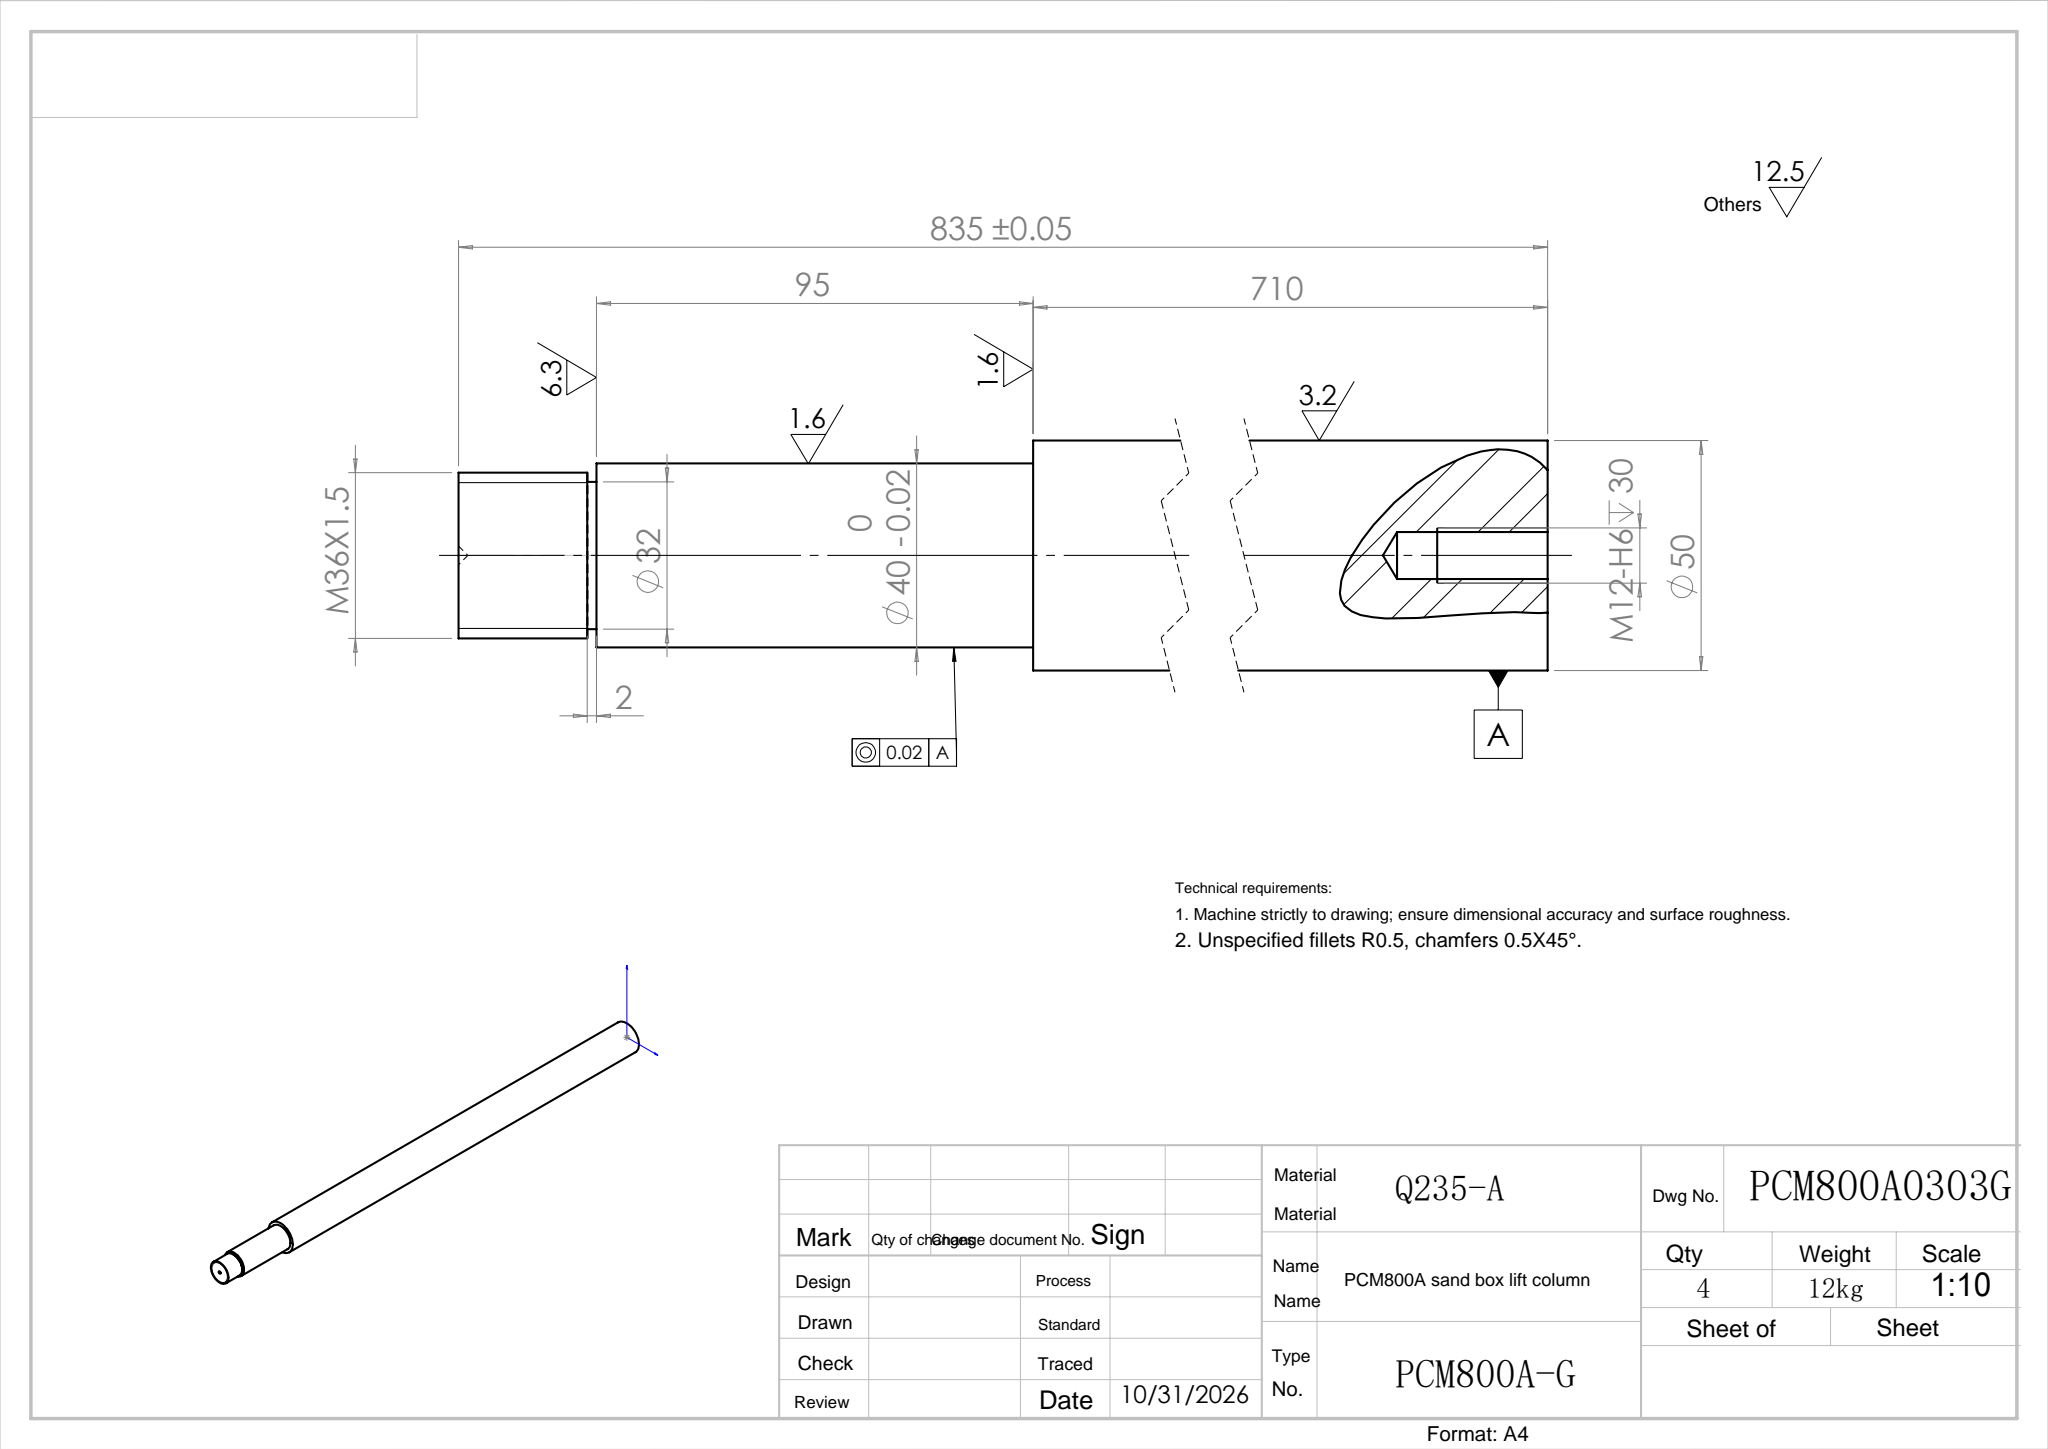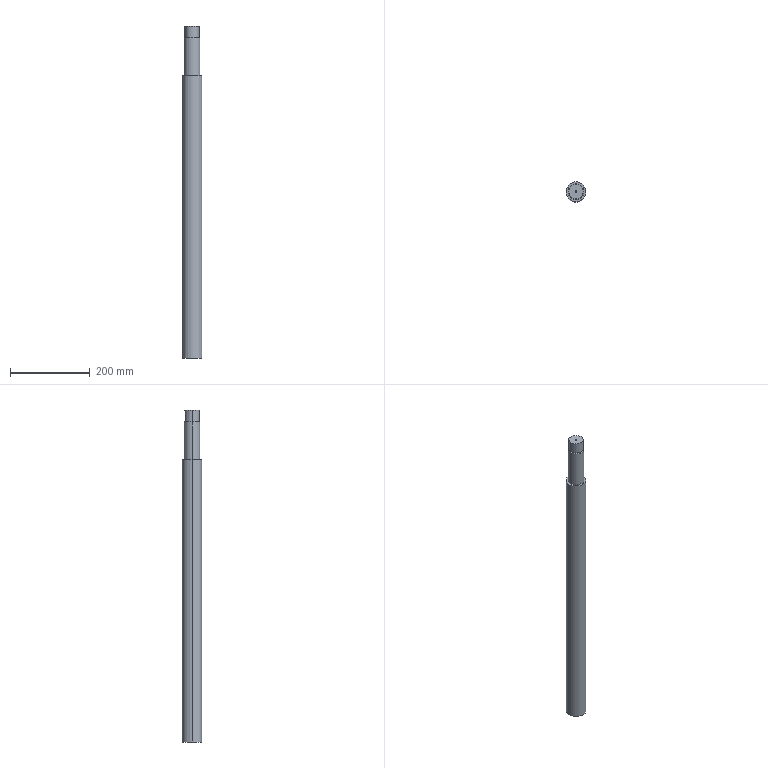Part | SolidWorks | features Boss 2, Extrusion 1, HoleWzd 1, ICE 1, RevCut 1 | 1 solid | 19 faces | box 50 x 50 x 835 mm | volume 1540803 mm3 | cylinder 10 | plane 5 | cone 4 | commonest cylinder face diameters 10.2 x2 32 x2 36 x2 40 x2 50 x2
STEP:
#1=CARTESIAN_POINT('',(18.,0.,835.));
#2=VERTEX_POINT('',#1);
#3=CARTESIAN_POINT('',(-18.,0.,835.));
#4=VERTEX_POINT('',#3);
#5=CARTESIAN_POINT('',(0.,0.,835.));
#6=DIRECTION('',(0.,0.,1.));
#7=DIRECTION('',(1.,0.,0.));
#8=AXIS2_PLACEMENT_3D('',#5,#6,#7);
#9=CIRCLE('',#8,18.);
#10=EDGE_CURVE('',#2,#4,#9,.T.);
#11=ORIENTED_EDGE('',*,*,#10,.F.);
#12=CARTESIAN_POINT('',(18.,0.,807.));
#13=VERTEX_POINT('',#12);
#14=CARTESIAN_POINT('',(18.,0.,835.));
#15=DIRECTION('',(0.,0.,-1.));
#16=VECTOR('',#15,1000.);
#17=LINE('',#14,#16);
#18=EDGE_CURVE('',#2,#13,#17,.T.);
#19=ORIENTED_EDGE('',*,*,#18,.T.);
#20=CARTESIAN_POINT('',(-18.,0.,807.));
#21=VERTEX_POINT('',#20);
#22=CARTESIAN_POINT('',(0.,0.,807.));
#23=DIRECTION('',(0.,0.,1.));
#24=DIRECTION('',(1.,0.,0.));
#25=AXIS2_PLACEMENT_3D('',#22,#23,#24);
#26=CIRCLE('',#25,18.);
#27=EDGE_CURVE('',#13,#21,#26,.T.);
#28=ORIENTED_EDGE('',*,*,#27,.T.);
#29=CARTESIAN_POINT('',(-18.,0.,835.));
#30=DIRECTION('',(0.,0.,-1.));
#31=VECTOR('',#30,1000.);
#32=LINE('',#29,#31);
#33=EDGE_CURVE('',#4,#21,#32,.T.);
#34=ORIENTED_EDGE('',*,*,#33,.F.);
#35=EDGE_LOOP('',(#11,#19,#28,#34));
#36=FACE_OUTER_BOUND('',#35,.T.);
#37=CARTESIAN_POINT('',(0.,0.,835.));
#38=DIRECTION('',(0.,0.,-1.));
#39=DIRECTION('',(-1.,0.,0.));
#40=AXIS2_PLACEMENT_3D('',#37,#38,#39);
#41=CYLINDRICAL_SURFACE('',#40,18.);
#42=ADVANCED_FACE('',(#36),#41,.T.);
#43=CARTESIAN_POINT('',(0.,0.,833.));
#44=VERTEX_POINT('',#43);
#45=CARTESIAN_POINT('',(2.,0.,835.));
#46=VERTEX_POINT('',#45);
#47=CARTESIAN_POINT('',(0.,0.,833.));
#48=DIRECTION('',(0.7071,0.,0.7071));
#49=VECTOR('',#48,1000.);
#50=LINE('',#47,#49);
#51=EDGE_CURVE('',#44,#46,#50,.T.);
#52=ORIENTED_EDGE('',*,*,#51,.F.);
#53=CARTESIAN_POINT('',(-2.,0.,835.));
#54=VERTEX_POINT('',#53);
#55=CARTESIAN_POINT('',(0.,0.,833.));
#56=DIRECTION('',(-0.7071,0.,0.7071));
#57=VECTOR('',#56,1000.);
#58=LINE('',#55,#57);
#59=EDGE_CURVE('',#44,#54,#58,.T.);
#60=ORIENTED_EDGE('',*,*,#59,.T.);
#61=CARTESIAN_POINT('',(0.,0.,835.));
#62=DIRECTION('',(0.,0.,1.));
#63=DIRECTION('',(1.,0.,0.));
#64=AXIS2_PLACEMENT_3D('',#61,#62,#63);
#65=CIRCLE('',#64,2.);
#66=EDGE_CURVE('',#54,#46,#65,.T.);
#67=ORIENTED_EDGE('',*,*,#66,.T.);
#68=EDGE_LOOP('',(#52,#60,#67));
#69=FACE_OUTER_BOUND('',#68,.T.);
#70=CARTESIAN_POINT('',(0.,0.,1833.));
#71=DIRECTION('',(0.,0.,1.));
#72=DIRECTION('',(1.,0.,0.));
#73=AXIS2_PLACEMENT_3D('',#70,#71,#72);
#74=CONICAL_SURFACE('',#73,1000.,0.7854);
#75=ADVANCED_FACE('',(#69),#74,.F.);
#76=CARTESIAN_POINT('',(16.,0.,807.));
#77=VERTEX_POINT('',#76);
#78=CARTESIAN_POINT('',(-16.,0.,807.));
#79=VERTEX_POINT('',#78);
#80=CARTESIAN_POINT('',(0.,0.,807.));
#81=DIRECTION('',(0.,0.,1.));
#82=DIRECTION('',(1.,0.,0.));
#83=AXIS2_PLACEMENT_3D('',#80,#81,#82);
#84=CIRCLE('',#83,16.);
#85=EDGE_CURVE('',#77,#79,#84,.T.);
#86=ORIENTED_EDGE('',*,*,#85,.F.);
#87=CARTESIAN_POINT('',(16.,0.,805.));
#88=VERTEX_POINT('',#87);
#89=CARTESIAN_POINT('',(16.,0.,807.));
#90=DIRECTION('',(0.,0.,-1.));
#91=VECTOR('',#90,1000.);
#92=LINE('',#89,#91);
#93=EDGE_CURVE('',#77,#88,#92,.T.);
#94=ORIENTED_EDGE('',*,*,#93,.T.);
#95=CARTESIAN_POINT('',(-16.,0.,805.));
#96=VERTEX_POINT('',#95);
#97=CARTESIAN_POINT('',(0.,0.,805.));
#98=DIRECTION('',(0.,0.,1.));
#99=DIRECTION('',(1.,0.,0.));
#100=AXIS2_PLACEMENT_3D('',#97,#98,#99);
#101=CIRCLE('',#100,16.);
#102=EDGE_CURVE('',#88,#96,#101,.T.);
#103=ORIENTED_EDGE('',*,*,#102,.T.);
#104=CARTESIAN_POINT('',(-16.,0.,807.));
#105=DIRECTION('',(0.,0.,-1.));
#106=VECTOR('',#105,1000.);
#107=LINE('',#104,#106);
#108=EDGE_CURVE('',#79,#96,#107,.T.);
#109=ORIENTED_EDGE('',*,*,#108,.F.);
#110=EDGE_LOOP('',(#86,#94,#103,#109));
#111=FACE_OUTER_BOUND('',#110,.T.);
#112=CARTESIAN_POINT('',(0.,0.,807.));
#113=DIRECTION('',(0.,0.,-1.));
#114=DIRECTION('',(-1.,0.,0.));
#115=AXIS2_PLACEMENT_3D('',#112,#113,#114);
#116=CYLINDRICAL_SURFACE('',#115,16.);
#117=ADVANCED_FACE('',(#111),#116,.T.);
#118=CARTESIAN_POINT('',(5.1,0.,32.75));
#119=VERTEX_POINT('',#118);
#120=CARTESIAN_POINT('',(-5.1,0.,32.75));
#121=VERTEX_POINT('',#120);
#122=CARTESIAN_POINT('',(0.,0.,32.75));
#123=DIRECTION('',(0.,0.,-1.));
#124=DIRECTION('',(-1.,0.,0.));
#125=AXIS2_PLACEMENT_3D('',#122,#123,#124);
#126=CIRCLE('',#125,5.1);
#127=EDGE_CURVE('',#119,#121,#126,.T.);
#128=ORIENTED_EDGE('',*,*,#127,.F.);
#129=CARTESIAN_POINT('',(5.1,0.,0.));
#130=VERTEX_POINT('',#129);
#131=CARTESIAN_POINT('',(5.1,0.,0.));
#132=DIRECTION('',(0.,0.,-1.));
#133=VECTOR('',#132,1000.);
#134=LINE('',#131,#133);
#135=EDGE_CURVE('',#119,#130,#134,.T.);
#136=ORIENTED_EDGE('',*,*,#135,.T.);
#137=CARTESIAN_POINT('',(-5.1,0.,0.));
#138=VERTEX_POINT('',#137);
#139=CARTESIAN_POINT('',(0.,0.,0.));
#140=DIRECTION('',(0.,0.,-1.));
#141=DIRECTION('',(-1.,0.,0.));
#142=AXIS2_PLACEMENT_3D('',#139,#140,#141);
#143=CIRCLE('',#142,5.1);
#144=EDGE_CURVE('',#130,#138,#143,.T.);
#145=ORIENTED_EDGE('',*,*,#144,.T.);
#146=CARTESIAN_POINT('',(-5.1,0.,0.));
#147=DIRECTION('',(0.,0.,-1.));
#148=VECTOR('',#147,1000.);
#149=LINE('',#146,#148);
#150=EDGE_CURVE('',#121,#138,#149,.T.);
#151=ORIENTED_EDGE('',*,*,#150,.F.);
#152=EDGE_LOOP('',(#128,#136,#145,#151));
#153=FACE_OUTER_BOUND('',#152,.T.);
#154=CARTESIAN_POINT('',(0.,0.,0.));
#155=DIRECTION('',(0.,0.,-1.));
#156=DIRECTION('',(-1.,0.,0.));
#157=AXIS2_PLACEMENT_3D('',#154,#155,#156);
#158=CYLINDRICAL_SURFACE('',#157,5.1);
#159=ADVANCED_FACE('',(#153),#158,.F.);
#160=CARTESIAN_POINT('',(0.,0.,35.814));
#161=VERTEX_POINT('',#160);
#162=CARTESIAN_POINT('',(-5.1,0.,32.75));
#163=DIRECTION('',(-0.8572,0.,-0.515));
#164=VECTOR('',#163,1000.);
#165=LINE('',#162,#164);
#166=EDGE_CURVE('',#161,#121,#165,.T.);
#167=ORIENTED_EDGE('',*,*,#166,.F.);
#168=CARTESIAN_POINT('',(5.1,0.,32.75));
#169=DIRECTION('',(0.8572,0.,-0.515));
#170=VECTOR('',#169,1000.);
#171=LINE('',#168,#170);
#172=EDGE_CURVE('',#161,#119,#171,.T.);
#173=ORIENTED_EDGE('',*,*,#172,.T.);
#174=ORIENTED_EDGE('',*,*,#127,.T.);
#175=EDGE_LOOP('',(#167,#173,#174));
#176=FACE_OUTER_BOUND('',#175,.T.);
#177=CARTESIAN_POINT('',(0.,0.,32.75));
#178=DIRECTION('',(0.,0.,-1.));
#179=DIRECTION('',(-1.,0.,0.));
#180=AXIS2_PLACEMENT_3D('',#177,#178,#179);
#181=CONICAL_SURFACE('',#180,5.1,1.03);
#182=ADVANCED_FACE('',(#176),#181,.F.);
#183=CARTESIAN_POINT('',(20.,0.,805.));
#184=VERTEX_POINT('',#183);
#185=CARTESIAN_POINT('',(-20.,0.,805.));
#186=VERTEX_POINT('',#185);
#187=CARTESIAN_POINT('',(0.,0.,805.));
#188=DIRECTION('',(0.,0.,1.));
#189=DIRECTION('',(1.,0.,0.));
#190=AXIS2_PLACEMENT_3D('',#187,#188,#189);
#191=CIRCLE('',#190,20.);
#192=EDGE_CURVE('',#184,#186,#191,.T.);
#193=ORIENTED_EDGE('',*,*,#192,.F.);
#194=CARTESIAN_POINT('',(20.,0.,710.));
#195=VERTEX_POINT('',#194);
#196=CARTESIAN_POINT('',(20.,0.,805.));
#197=DIRECTION('',(0.,0.,-1.));
#198=VECTOR('',#197,1000.);
#199=LINE('',#196,#198);
#200=EDGE_CURVE('',#184,#195,#199,.T.);
#201=ORIENTED_EDGE('',*,*,#200,.T.);
#202=CARTESIAN_POINT('',(-20.,0.,710.));
#203=VERTEX_POINT('',#202);
#204=CARTESIAN_POINT('',(0.,0.,710.));
#205=DIRECTION('',(0.,0.,1.));
#206=DIRECTION('',(1.,0.,0.));
#207=AXIS2_PLACEMENT_3D('',#204,#205,#206);
#208=CIRCLE('',#207,20.);
#209=EDGE_CURVE('',#195,#203,#208,.T.);
#210=ORIENTED_EDGE('',*,*,#209,.T.);
#211=CARTESIAN_POINT('',(-20.,0.,805.));
#212=DIRECTION('',(0.,0.,-1.));
#213=VECTOR('',#212,1000.);
#214=LINE('',#211,#213);
#215=EDGE_CURVE('',#186,#203,#214,.T.);
#216=ORIENTED_EDGE('',*,*,#215,.F.);
#217=EDGE_LOOP('',(#193,#201,#210,#216));
#218=FACE_OUTER_BOUND('',#217,.T.);
#219=CARTESIAN_POINT('',(0.,0.,805.));
#220=DIRECTION('',(0.,0.,-1.));
#221=DIRECTION('',(-1.,0.,0.));
#222=AXIS2_PLACEMENT_3D('',#219,#220,#221);
#223=CYLINDRICAL_SURFACE('',#222,20.);
#224=ADVANCED_FACE('',(#218),#223,.T.);
#225=CARTESIAN_POINT('',(25.,0.,710.));
#226=VERTEX_POINT('',#225);
#227=CARTESIAN_POINT('',(-25.,0.,710.));
#228=VERTEX_POINT('',#227);
#229=CARTESIAN_POINT('',(0.,0.,710.));
#230=DIRECTION('',(0.,0.,1.));
#231=DIRECTION('',(1.,0.,0.));
#232=AXIS2_PLACEMENT_3D('',#229,#230,#231);
#233=CIRCLE('',#232,25.);
#234=EDGE_CURVE('',#226,#228,#233,.T.);
#235=ORIENTED_EDGE('',*,*,#234,.F.);
#236=CARTESIAN_POINT('',(25.,0.,0.));
#237=VERTEX_POINT('',#236);
#238=CARTESIAN_POINT('',(25.,0.,710.));
#239=DIRECTION('',(0.,0.,-1.));
#240=VECTOR('',#239,1000.);
#241=LINE('',#238,#240);
#242=EDGE_CURVE('',#226,#237,#241,.T.);
#243=ORIENTED_EDGE('',*,*,#242,.T.);
#244=CARTESIAN_POINT('',(-25.,0.,0.));
#245=VERTEX_POINT('',#244);
#246=CARTESIAN_POINT('',(0.,0.,0.));
#247=DIRECTION('',(0.,0.,1.));
#248=DIRECTION('',(1.,0.,0.));
#249=AXIS2_PLACEMENT_3D('',#246,#247,#248);
#250=CIRCLE('',#249,25.);
#251=EDGE_CURVE('',#237,#245,#250,.T.);
#252=ORIENTED_EDGE('',*,*,#251,.T.);
#253=CARTESIAN_POINT('',(-25.,0.,710.));
#254=DIRECTION('',(0.,0.,-1.));
#255=VECTOR('',#254,1000.);
#256=LINE('',#253,#255);
#257=EDGE_CURVE('',#228,#245,#256,.T.);
#258=ORIENTED_EDGE('',*,*,#257,.F.);
#259=EDGE_LOOP('',(#235,#243,#252,#258));
#260=FACE_OUTER_BOUND('',#259,.T.);
#261=CARTESIAN_POINT('',(0.,0.,710.));
#262=DIRECTION('',(0.,0.,-1.));
#263=DIRECTION('',(-1.,0.,0.));
#264=AXIS2_PLACEMENT_3D('',#261,#262,#263);
#265=CYLINDRICAL_SURFACE('',#264,25.);
#266=ADVANCED_FACE('',(#260),#265,.T.);
#267=CARTESIAN_POINT('',(0.,0.,805.));
#268=DIRECTION('',(0.,0.,1.));
#269=DIRECTION('',(1.,0.,0.));
#270=AXIS2_PLACEMENT_3D('',#267,#268,#269);
#271=CIRCLE('',#270,20.);
#272=EDGE_CURVE('',#186,#184,#271,.T.);
#273=ORIENTED_EDGE('',*,*,#272,.T.);
#274=ORIENTED_EDGE('',*,*,#192,.T.);
#275=EDGE_LOOP('',(#273,#274));
#276=FACE_OUTER_BOUND('',#275,.T.);
#277=CARTESIAN_POINT('',(0.,0.,805.));
#278=DIRECTION('',(0.,0.,1.));
#279=DIRECTION('',(1.,0.,0.));
#280=AXIS2_PLACEMENT_3D('',#277,#278,#279);
#281=CIRCLE('',#280,16.);
#282=EDGE_CURVE('',#96,#88,#281,.T.);
#283=ORIENTED_EDGE('',*,*,#282,.F.);
#284=ORIENTED_EDGE('',*,*,#102,.F.);
#285=EDGE_LOOP('',(#283,#284));
#286=FACE_BOUND('',#285,.T.);
#287=CARTESIAN_POINT('',(0.,0.,805.));
#288=DIRECTION('',(0.,0.,1.));
#289=DIRECTION('',(1.,0.,0.));
#290=AXIS2_PLACEMENT_3D('',#287,#288,#289);
#291=PLANE('',#290);
#292=ADVANCED_FACE('',(#276,#286),#291,.T.);
#293=CARTESIAN_POINT('',(0.,0.,710.));
#294=DIRECTION('',(0.,0.,1.));
#295=DIRECTION('',(1.,0.,0.));
#296=AXIS2_PLACEMENT_3D('',#293,#294,#295);
#297=CIRCLE('',#296,25.);
#298=EDGE_CURVE('',#228,#226,#297,.T.);
#299=ORIENTED_EDGE('',*,*,#298,.T.);
#300=ORIENTED_EDGE('',*,*,#234,.T.);
#301=EDGE_LOOP('',(#299,#300));
#302=FACE_OUTER_BOUND('',#301,.T.);
#303=CARTESIAN_POINT('',(0.,0.,710.));
#304=DIRECTION('',(0.,0.,1.));
#305=DIRECTION('',(1.,0.,0.));
#306=AXIS2_PLACEMENT_3D('',#303,#304,#305);
#307=CIRCLE('',#306,20.);
#308=EDGE_CURVE('',#203,#195,#307,.T.);
#309=ORIENTED_EDGE('',*,*,#308,.F.);
#310=ORIENTED_EDGE('',*,*,#209,.F.);
#311=EDGE_LOOP('',(#309,#310));
#312=FACE_BOUND('',#311,.T.);
#313=CARTESIAN_POINT('',(0.,0.,710.));
#314=DIRECTION('',(0.,0.,1.));
#315=DIRECTION('',(1.,0.,0.));
#316=AXIS2_PLACEMENT_3D('',#313,#314,#315);
#317=PLANE('',#316);
#318=ADVANCED_FACE('',(#302,#312),#317,.T.);
#319=ORIENTED_EDGE('',*,*,#242,.F.);
#320=ORIENTED_EDGE('',*,*,#298,.F.);
#321=ORIENTED_EDGE('',*,*,#257,.T.);
#322=CARTESIAN_POINT('',(0.,0.,0.));
#323=DIRECTION('',(0.,0.,1.));
#324=DIRECTION('',(1.,0.,0.));
#325=AXIS2_PLACEMENT_3D('',#322,#323,#324);
#326=CIRCLE('',#325,25.);
#327=EDGE_CURVE('',#245,#237,#326,.T.);
#328=ORIENTED_EDGE('',*,*,#327,.T.);
#329=EDGE_LOOP('',(#319,#320,#321,#328));
#330=FACE_OUTER_BOUND('',#329,.T.);
#331=CARTESIAN_POINT('',(0.,0.,710.));
#332=DIRECTION('',(0.,0.,-1.));
#333=DIRECTION('',(-1.,0.,0.));
#334=AXIS2_PLACEMENT_3D('',#331,#332,#333);
#335=CYLINDRICAL_SURFACE('',#334,25.);
#336=ADVANCED_FACE('',(#330),#335,.T.);
#337=CARTESIAN_POINT('',(0.,0.,0.));
#338=DIRECTION('',(0.,0.,-1.));
#339=DIRECTION('',(-1.,0.,0.));
#340=AXIS2_PLACEMENT_3D('',#337,#338,#339);
#341=CIRCLE('',#340,5.1);
#342=EDGE_CURVE('',#138,#130,#341,.T.);
#343=ORIENTED_EDGE('',*,*,#342,.F.);
#344=ORIENTED_EDGE('',*,*,#144,.F.);
#345=EDGE_LOOP('',(#343,#344));
#346=FACE_BOUND('',#345,.T.);
#347=ORIENTED_EDGE('',*,*,#327,.F.);
#348=ORIENTED_EDGE('',*,*,#251,.F.);
#349=EDGE_LOOP('',(#347,#348));
#350=FACE_OUTER_BOUND('',#349,.T.);
#351=CARTESIAN_POINT('',(0.,0.,0.));
#352=DIRECTION('',(0.,0.,1.));
#353=DIRECTION('',(1.,0.,0.));
#354=AXIS2_PLACEMENT_3D('',#351,#352,#353);
#355=PLANE('',#354);
#356=ADVANCED_FACE('',(#346,#350),#355,.F.);
#357=ORIENTED_EDGE('',*,*,#200,.F.);
#358=ORIENTED_EDGE('',*,*,#272,.F.);
#359=ORIENTED_EDGE('',*,*,#215,.T.);
#360=ORIENTED_EDGE('',*,*,#308,.T.);
#361=EDGE_LOOP('',(#357,#358,#359,#360));
#362=FACE_OUTER_BOUND('',#361,.T.);
#363=CARTESIAN_POINT('',(0.,0.,805.));
#364=DIRECTION('',(0.,0.,-1.));
#365=DIRECTION('',(-1.,0.,0.));
#366=AXIS2_PLACEMENT_3D('',#363,#364,#365);
#367=CYLINDRICAL_SURFACE('',#366,20.);
#368=ADVANCED_FACE('',(#362),#367,.T.);
#369=ORIENTED_EDGE('',*,*,#172,.F.);
#370=ORIENTED_EDGE('',*,*,#166,.T.);
#371=CARTESIAN_POINT('',(0.,0.,32.75));
#372=DIRECTION('',(0.,0.,-1.));
#373=DIRECTION('',(-1.,0.,0.));
#374=AXIS2_PLACEMENT_3D('',#371,#372,#373);
#375=CIRCLE('',#374,5.1);
#376=EDGE_CURVE('',#121,#119,#375,.T.);
#377=ORIENTED_EDGE('',*,*,#376,.T.);
#378=EDGE_LOOP('',(#369,#370,#377));
#379=FACE_OUTER_BOUND('',#378,.T.);
#380=CARTESIAN_POINT('',(0.,0.,32.75));
#381=DIRECTION('',(0.,0.,-1.));
#382=DIRECTION('',(-1.,0.,0.));
#383=AXIS2_PLACEMENT_3D('',#380,#381,#382);
#384=CONICAL_SURFACE('',#383,5.1,1.03);
#385=ADVANCED_FACE('',(#379),#384,.F.);
#386=ORIENTED_EDGE('',*,*,#135,.F.);
#387=ORIENTED_EDGE('',*,*,#376,.F.);
#388=ORIENTED_EDGE('',*,*,#150,.T.);
#389=ORIENTED_EDGE('',*,*,#342,.T.);
#390=EDGE_LOOP('',(#386,#387,#388,#389));
#391=FACE_OUTER_BOUND('',#390,.T.);
#392=CARTESIAN_POINT('',(0.,0.,0.));
#393=DIRECTION('',(0.,0.,-1.));
#394=DIRECTION('',(-1.,0.,0.));
#395=AXIS2_PLACEMENT_3D('',#392,#393,#394);
#396=CYLINDRICAL_SURFACE('',#395,5.1);
#397=ADVANCED_FACE('',(#391),#396,.F.);
#398=CARTESIAN_POINT('',(0.,0.,807.));
#399=DIRECTION('',(0.,0.,1.));
#400=DIRECTION('',(1.,0.,0.));
#401=AXIS2_PLACEMENT_3D('',#398,#399,#400);
#402=CIRCLE('',#401,16.);
#403=EDGE_CURVE('',#79,#77,#402,.T.);
#404=ORIENTED_EDGE('',*,*,#403,.T.);
#405=ORIENTED_EDGE('',*,*,#85,.T.);
#406=EDGE_LOOP('',(#404,#405));
#407=FACE_BOUND('',#406,.T.);
#408=CARTESIAN_POINT('',(0.,0.,807.));
#409=DIRECTION('',(0.,0.,1.));
#410=DIRECTION('',(1.,0.,0.));
#411=AXIS2_PLACEMENT_3D('',#408,#409,#410);
#412=CIRCLE('',#411,18.);
#413=EDGE_CURVE('',#21,#13,#412,.T.);
#414=ORIENTED_EDGE('',*,*,#413,.F.);
#415=ORIENTED_EDGE('',*,*,#27,.F.);
#416=EDGE_LOOP('',(#414,#415));
#417=FACE_OUTER_BOUND('',#416,.T.);
#418=CARTESIAN_POINT('',(0.,0.,807.));
#419=DIRECTION('',(0.,0.,1.));
#420=DIRECTION('',(1.,0.,0.));
#421=AXIS2_PLACEMENT_3D('',#418,#419,#420);
#422=PLANE('',#421);
#423=ADVANCED_FACE('',(#407,#417),#422,.F.);
#424=ORIENTED_EDGE('',*,*,#93,.F.);
#425=ORIENTED_EDGE('',*,*,#403,.F.);
#426=ORIENTED_EDGE('',*,*,#108,.T.);
#427=ORIENTED_EDGE('',*,*,#282,.T.);
#428=EDGE_LOOP('',(#424,#425,#426,#427));
#429=FACE_OUTER_BOUND('',#428,.T.);
#430=CARTESIAN_POINT('',(0.,0.,807.));
#431=DIRECTION('',(0.,0.,-1.));
#432=DIRECTION('',(-1.,0.,0.));
#433=AXIS2_PLACEMENT_3D('',#430,#431,#432);
#434=CYLINDRICAL_SURFACE('',#433,16.);
#435=ADVANCED_FACE('',(#429),#434,.T.);
#436=ORIENTED_EDGE('',*,*,#59,.F.);
#437=ORIENTED_EDGE('',*,*,#51,.T.);
#438=CARTESIAN_POINT('',(0.,0.,835.));
#439=DIRECTION('',(0.,0.,1.));
#440=DIRECTION('',(1.,0.,0.));
#441=AXIS2_PLACEMENT_3D('',#438,#439,#440);
#442=CIRCLE('',#441,2.);
#443=EDGE_CURVE('',#46,#54,#442,.T.);
#444=ORIENTED_EDGE('',*,*,#443,.T.);
#445=EDGE_LOOP('',(#436,#437,#444));
#446=FACE_OUTER_BOUND('',#445,.T.);
#447=CARTESIAN_POINT('',(0.,0.,1833.));
#448=DIRECTION('',(0.,0.,1.));
#449=DIRECTION('',(1.,0.,0.));
#450=AXIS2_PLACEMENT_3D('',#447,#448,#449);
#451=CONICAL_SURFACE('',#450,1000.,0.7854);
#452=ADVANCED_FACE('',(#446),#451,.F.);
#453=CARTESIAN_POINT('',(0.,0.,835.));
#454=DIRECTION('',(0.,0.,1.));
#455=DIRECTION('',(1.,0.,0.));
#456=AXIS2_PLACEMENT_3D('',#453,#454,#455);
#457=CIRCLE('',#456,18.);
#458=EDGE_CURVE('',#4,#2,#457,.T.);
#459=ORIENTED_EDGE('',*,*,#458,.T.);
#460=ORIENTED_EDGE('',*,*,#10,.T.);
#461=EDGE_LOOP('',(#459,#460));
#462=FACE_OUTER_BOUND('',#461,.T.);
#463=ORIENTED_EDGE('',*,*,#443,.F.);
#464=ORIENTED_EDGE('',*,*,#66,.F.);
#465=EDGE_LOOP('',(#463,#464));
#466=FACE_BOUND('',#465,.T.);
#467=CARTESIAN_POINT('',(0.,0.,835.));
#468=DIRECTION('',(0.,0.,1.));
#469=DIRECTION('',(1.,0.,0.));
#470=AXIS2_PLACEMENT_3D('',#467,#468,#469);
#471=PLANE('',#470);
#472=ADVANCED_FACE('',(#462,#466),#471,.T.);
#473=ORIENTED_EDGE('',*,*,#18,.F.);
#474=ORIENTED_EDGE('',*,*,#458,.F.);
#475=ORIENTED_EDGE('',*,*,#33,.T.);
#476=ORIENTED_EDGE('',*,*,#413,.T.);
#477=EDGE_LOOP('',(#473,#474,#475,#476));
#478=FACE_OUTER_BOUND('',#477,.T.);
#479=CARTESIAN_POINT('',(0.,0.,835.));
#480=DIRECTION('',(0.,0.,-1.));
#481=DIRECTION('',(-1.,0.,0.));
#482=AXIS2_PLACEMENT_3D('',#479,#480,#481);
#483=CYLINDRICAL_SURFACE('',#482,18.);
#484=ADVANCED_FACE('',(#478),#483,.T.);
#485=CLOSED_SHELL('',(#42,#75,#117,#159,#182,#224,#266,#292,#318,#336,#356,#368,#385,#397,#423,#435,#452,#472,#484));
#486=MANIFOLD_SOLID_BREP('',#485);
#487=CARTESIAN_POINT('',(0.,0.,0.));
#488=DIRECTION('',(0.,0.,1.));
#489=DIRECTION('',(1.,0.,0.));
#490=AXIS2_PLACEMENT_3D('',#487,#488,#489);
#491=(LENGTH_UNIT()NAMED_UNIT(*)SI_UNIT(.MILLI.,.METRE.));
#492=UNCERTAINTY_MEASURE_WITH_UNIT(LENGTH_MEASURE(0.00001),#491,'','');
#493=(NAMED_UNIT(*)PLANE_ANGLE_UNIT()SI_UNIT($,.RADIAN.));
#494=(NAMED_UNIT(*)SI_UNIT($,.STERADIAN.)SOLID_ANGLE_UNIT());
#495=(GEOMETRIC_REPRESENTATION_CONTEXT(3)GLOBAL_UNCERTAINTY_ASSIGNED_CONTEXT((#492))GLOBAL_UNIT_ASSIGNED_CONTEXT((#491,#493,#494))REPRESENTATION_CONTEXT('',''));
#496=ADVANCED_BREP_SHAPE_REPRESENTATION('',(#486,#490),#495);